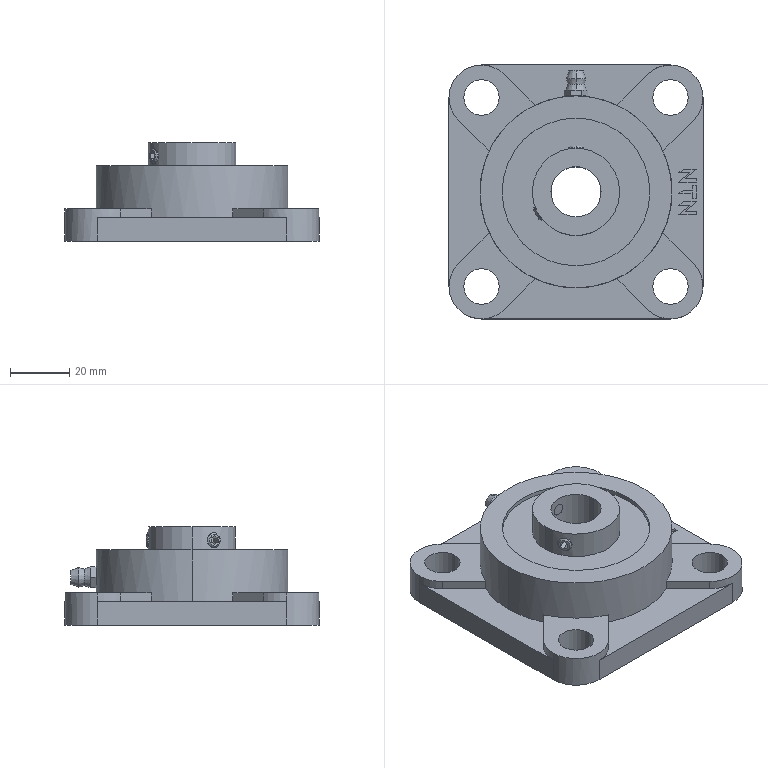Part | STEP file | Produce dryer-ucf203 | 2 solids | 146 faces | box 86 x 86 x 33.3 mm | volume 92180 mm3 | plane 95 | cylinder 41 | cone 10 | commonest cylinder face diameters 22 x12 12 x8 4.019 x5 5 x4 29.6 x4 50 x4